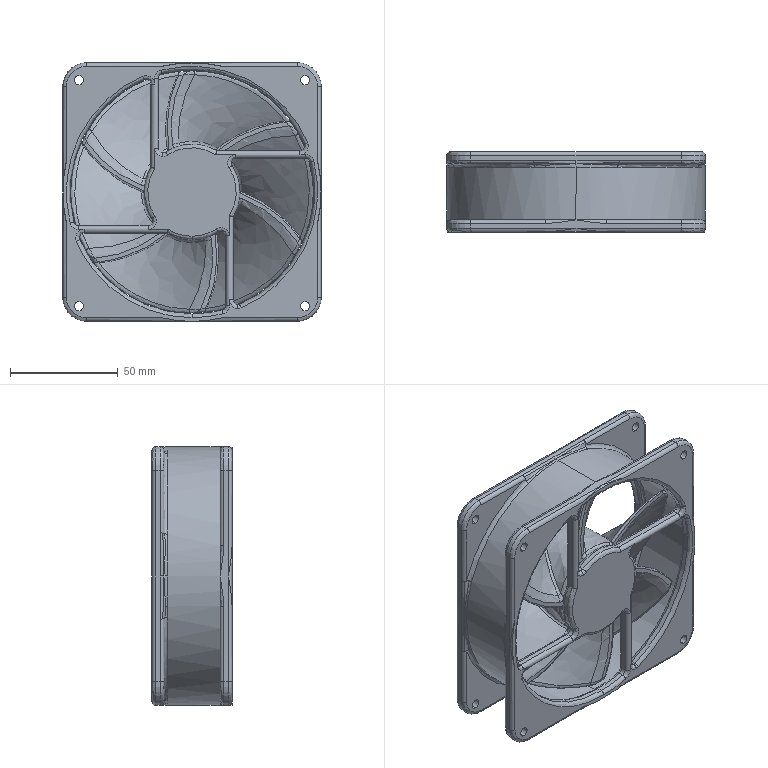Part | SolidWorks | features AEMSimFeature 1 | 1 solid | 407 faces | box 120.002 x 37.222 x 120.002 mm | volume 118437 mm3 | spline 258 | cylinder 103 | plane 46 | commonest cylinder face diameters 3.333 x36 4.444 x18 4.3 x16 22.222 x8 113.333 x7 120 x7